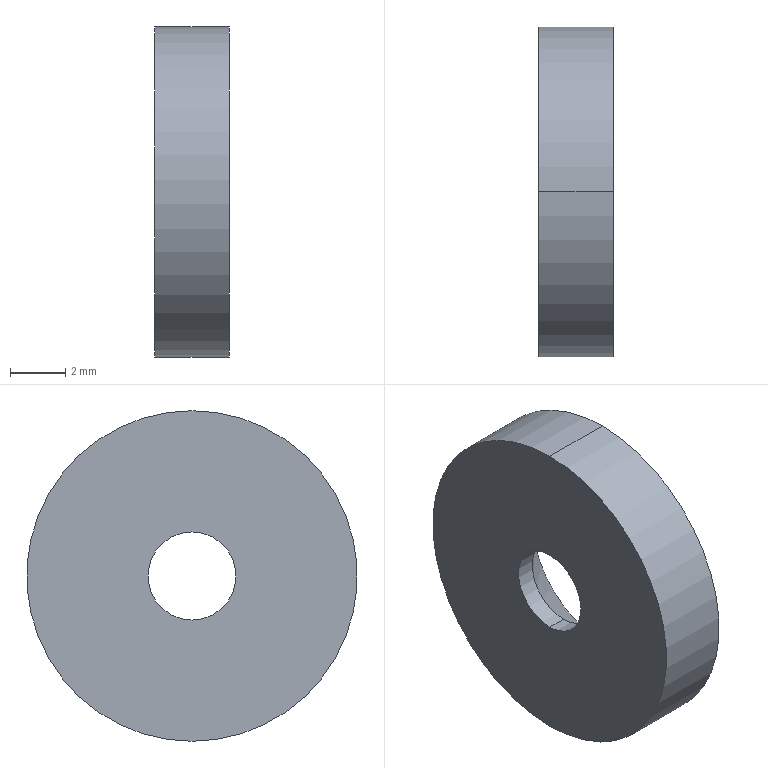Part | STEP file | NdFeB round magnet D12X3 with 3mm hole | 1 solid | 8 faces | box 2.7 x 12 x 12 mm | volume 255.164 mm3 | cylinder 4 | cone 2 | plane 2 | commonest cylinder face diameters 3.2 x2 12 x2
STEP:
#1=CARTESIAN_POINT('',(0.,0.,0.));
#2=DIRECTION('',(0.,0.,1.));
#3=DIRECTION('',(1.,0.,0.));
#4=AXIS2_PLACEMENT_3D('',#1,#2,#3);
#5=CARTESIAN_POINT('',(0.7,0.,-1.6));
#6=VERTEX_POINT('',#5);
#7=CARTESIAN_POINT('',(2.7,0.,-3.6));
#8=VERTEX_POINT('',#7);
#9=CARTESIAN_POINT('',(0.7,0.,-1.6));
#10=DIRECTION('',(0.7071,0.,-0.7071));
#11=VECTOR('',#10,1.);
#12=LINE('',#9,#11);
#13=CARTESIAN_POINT('',(0.7,0.,0.));
#14=DIRECTION('',(1.,0.,0.));
#15=DIRECTION('',(0.,0.,-1.));
#16=AXIS2_PLACEMENT_3D('',#13,#14,#15);
#17=CONICAL_SURFACE('',#16,1.6,0.7854);
#18=CARTESIAN_POINT('',(6.283,0.));
#19=DIRECTION('',(0.,1.));
#20=VECTOR('',#19,1.);
#21=LINE('',#18,#20);
#22=(GEOMETRIC_REPRESENTATION_CONTEXT(2)PARAMETRIC_REPRESENTATION_CONTEXT()REPRESENTATION_CONTEXT('',''));
#23=DEFINITIONAL_REPRESENTATION('',(#21),#22);
#24=PCURVE('',#17,#23);
#25=CARTESIAN_POINT('',(0.7,0.,0.));
#26=DIRECTION('',(1.,0.,0.));
#27=DIRECTION('',(0.,0.,-1.));
#28=AXIS2_PLACEMENT_3D('',#25,#26,#27);
#29=CONICAL_SURFACE('',#28,1.6,0.7854);
#30=CARTESIAN_POINT('',(0.,0.));
#31=DIRECTION('',(0.,1.));
#32=VECTOR('',#31,1.);
#33=LINE('',#30,#32);
#34=(GEOMETRIC_REPRESENTATION_CONTEXT(2)PARAMETRIC_REPRESENTATION_CONTEXT()REPRESENTATION_CONTEXT('',''));
#35=DEFINITIONAL_REPRESENTATION('',(#33),#34);
#36=PCURVE('',#29,#35);
#37=SURFACE_CURVE('',#12,(#24,#36),.PCURVE_S1.);
#38=EDGE_CURVE('',#6,#8,#37,.T.);
#39=ORIENTED_EDGE('',*,*,#38,.T.);
#40=CARTESIAN_POINT('',(2.7,0.,3.6));
#41=VERTEX_POINT('',#40);
#42=CARTESIAN_POINT('',(2.7,0.,0.));
#43=DIRECTION('',(-1.,0.,0.));
#44=DIRECTION('',(0.,0.,-1.));
#45=AXIS2_PLACEMENT_3D('',#42,#43,#44);
#46=CIRCLE('',#45,3.6);
#47=CARTESIAN_POINT('',(6.283,2.));
#48=DIRECTION('',(-1.,0.));
#49=VECTOR('',#48,1.);
#50=LINE('',#47,#49);
#51=(GEOMETRIC_REPRESENTATION_CONTEXT(2)PARAMETRIC_REPRESENTATION_CONTEXT()REPRESENTATION_CONTEXT('',''));
#52=DEFINITIONAL_REPRESENTATION('',(#50),#51);
#53=PCURVE('',#17,#52);
#54=CARTESIAN_POINT('',(2.7,0.,0.));
#55=DIRECTION('',(1.,0.,0.));
#56=DIRECTION('',(0.,0.,-1.));
#57=AXIS2_PLACEMENT_3D('',#54,#55,#56);
#58=PLANE('',#57);
#59=CARTESIAN_POINT('',(3.6,0.));
#60=CARTESIAN_POINT('',(3.6,-6.235));
#61=CARTESIAN_POINT('',(-1.8,-3.118));
#62=CARTESIAN_POINT('',(-7.2,0.));
#63=CARTESIAN_POINT('',(-1.8,3.118));
#64=CARTESIAN_POINT('',(3.6,6.235));
#65=CARTESIAN_POINT('',(3.6,0.));
#66=(BOUNDED_CURVE()B_SPLINE_CURVE(2,(#59,#60,#61,#62,#63,#64,#65),.UNSPECIFIED.,.T.,.F.)B_SPLINE_CURVE_WITH_KNOTS((1,2,2,2,2,1),(-2.094,0.,2.094,4.189,6.283,8.378),.UNSPECIFIED.)CURVE()GEOMETRIC_REPRESENTATION_ITEM()RATIONAL_B_SPLINE_CURVE((1.,0.5,1.,0.5,1.,0.5,1.))REPRESENTATION_ITEM(''));
#67=(GEOMETRIC_REPRESENTATION_CONTEXT(2)PARAMETRIC_REPRESENTATION_CONTEXT()REPRESENTATION_CONTEXT('',''));
#68=DEFINITIONAL_REPRESENTATION('',(#66),#67);
#69=PCURVE('',#58,#68);
#70=SURFACE_CURVE('',#46,(#53,#69),.PCURVE_S1.);
#71=EDGE_CURVE('',#8,#41,#70,.T.);
#72=ORIENTED_EDGE('',*,*,#71,.T.);
#73=CARTESIAN_POINT('',(0.7,0.,1.6));
#74=VERTEX_POINT('',#73);
#75=CARTESIAN_POINT('',(0.7,0.,1.6));
#76=DIRECTION('',(0.7071,0.,0.7071));
#77=VECTOR('',#76,1.);
#78=LINE('',#75,#77);
#79=CARTESIAN_POINT('',(3.142,0.));
#80=DIRECTION('',(0.,1.));
#81=VECTOR('',#80,1.);
#82=LINE('',#79,#81);
#83=(GEOMETRIC_REPRESENTATION_CONTEXT(2)PARAMETRIC_REPRESENTATION_CONTEXT()REPRESENTATION_CONTEXT('',''));
#84=DEFINITIONAL_REPRESENTATION('',(#82),#83);
#85=PCURVE('',#17,#84);
#86=CARTESIAN_POINT('',(3.142,0.));
#87=DIRECTION('',(0.,1.));
#88=VECTOR('',#87,1.);
#89=LINE('',#86,#88);
#90=(GEOMETRIC_REPRESENTATION_CONTEXT(2)PARAMETRIC_REPRESENTATION_CONTEXT()REPRESENTATION_CONTEXT('',''));
#91=DEFINITIONAL_REPRESENTATION('',(#89),#90);
#92=PCURVE('',#29,#91);
#93=SURFACE_CURVE('',#78,(#85,#92),.PCURVE_S1.);
#94=EDGE_CURVE('',#74,#41,#93,.T.);
#95=ORIENTED_EDGE('',*,*,#94,.F.);
#96=CARTESIAN_POINT('',(0.7,0.,0.));
#97=DIRECTION('',(1.,0.,0.));
#98=DIRECTION('',(0.,0.,-1.));
#99=AXIS2_PLACEMENT_3D('',#96,#97,#98);
#100=CIRCLE('',#99,1.6);
#101=CARTESIAN_POINT('',(0.,0.));
#102=DIRECTION('',(1.,0.));
#103=VECTOR('',#102,1.);
#104=LINE('',#101,#103);
#105=(GEOMETRIC_REPRESENTATION_CONTEXT(2)PARAMETRIC_REPRESENTATION_CONTEXT()REPRESENTATION_CONTEXT('',''));
#106=DEFINITIONAL_REPRESENTATION('',(#104),#105);
#107=PCURVE('',#17,#106);
#108=CARTESIAN_POINT('',(2.7,0.,0.));
#109=DIRECTION('',(-1.,0.,0.));
#110=DIRECTION('',(0.,0.,1.));
#111=AXIS2_PLACEMENT_3D('',#108,#109,#110);
#112=CYLINDRICAL_SURFACE('',#111,1.6);
#113=CARTESIAN_POINT('',(9.425,2.));
#114=DIRECTION('',(-1.,0.));
#115=VECTOR('',#114,1.);
#116=LINE('',#113,#115);
#117=(GEOMETRIC_REPRESENTATION_CONTEXT(2)PARAMETRIC_REPRESENTATION_CONTEXT()REPRESENTATION_CONTEXT('',''));
#118=DEFINITIONAL_REPRESENTATION('',(#116),#117);
#119=PCURVE('',#112,#118);
#120=SURFACE_CURVE('',#100,(#107,#119),.PCURVE_S1.);
#121=EDGE_CURVE('',#74,#6,#120,.T.);
#122=ORIENTED_EDGE('',*,*,#121,.T.);
#123=EDGE_LOOP('',(#39,#72,#95,#122));
#124=FACE_BOUND('',#123,.F.);
#125=ADVANCED_FACE('',(#124),#17,.F.);
#126=CARTESIAN_POINT('',(0.,0.,1.6));
#127=VERTEX_POINT('',#126);
#128=CARTESIAN_POINT('',(2.7,0.,1.6));
#129=DIRECTION('',(-1.,0.,0.));
#130=VECTOR('',#129,1.);
#131=LINE('',#128,#130);
#132=CARTESIAN_POINT('',(6.283,0.));
#133=DIRECTION('',(0.,1.));
#134=VECTOR('',#133,1.);
#135=LINE('',#132,#134);
#136=(GEOMETRIC_REPRESENTATION_CONTEXT(2)PARAMETRIC_REPRESENTATION_CONTEXT()REPRESENTATION_CONTEXT('',''));
#137=DEFINITIONAL_REPRESENTATION('',(#135),#136);
#138=PCURVE('',#112,#137);
#139=CARTESIAN_POINT('',(2.7,0.,0.));
#140=DIRECTION('',(-1.,0.,0.));
#141=DIRECTION('',(0.,0.,1.));
#142=AXIS2_PLACEMENT_3D('',#139,#140,#141);
#143=CYLINDRICAL_SURFACE('',#142,1.6);
#144=CARTESIAN_POINT('',(0.,0.));
#145=DIRECTION('',(0.,1.));
#146=VECTOR('',#145,1.);
#147=LINE('',#144,#146);
#148=(GEOMETRIC_REPRESENTATION_CONTEXT(2)PARAMETRIC_REPRESENTATION_CONTEXT()REPRESENTATION_CONTEXT('',''));
#149=DEFINITIONAL_REPRESENTATION('',(#147),#148);
#150=PCURVE('',#143,#149);
#151=SURFACE_CURVE('',#131,(#138,#150),.PCURVE_S1.);
#152=EDGE_CURVE('',#74,#127,#151,.T.);
#153=ORIENTED_EDGE('',*,*,#152,.T.);
#154=CARTESIAN_POINT('',(0.,0.,-1.6));
#155=VERTEX_POINT('',#154);
#156=CARTESIAN_POINT('',(0.,0.,0.));
#157=DIRECTION('',(1.,0.,0.));
#158=DIRECTION('',(0.,0.,-1.));
#159=AXIS2_PLACEMENT_3D('',#156,#157,#158);
#160=CIRCLE('',#159,1.6);
#161=CARTESIAN_POINT('',(9.425,2.7));
#162=DIRECTION('',(-1.,0.));
#163=VECTOR('',#162,1.);
#164=LINE('',#161,#163);
#165=(GEOMETRIC_REPRESENTATION_CONTEXT(2)PARAMETRIC_REPRESENTATION_CONTEXT()REPRESENTATION_CONTEXT('',''));
#166=DEFINITIONAL_REPRESENTATION('',(#164),#165);
#167=PCURVE('',#112,#166);
#168=CARTESIAN_POINT('',(0.,0.,0.));
#169=DIRECTION('',(1.,0.,0.));
#170=DIRECTION('',(0.,0.,-1.));
#171=AXIS2_PLACEMENT_3D('',#168,#169,#170);
#172=PLANE('',#171);
#173=CARTESIAN_POINT('',(0.,0.));
#174=DIRECTION('',(1.,0.));
#175=AXIS2_PLACEMENT_2D('',#173,#174);
#176=CIRCLE('',#175,1.6);
#177=(GEOMETRIC_REPRESENTATION_CONTEXT(2)PARAMETRIC_REPRESENTATION_CONTEXT()REPRESENTATION_CONTEXT('',''));
#178=DEFINITIONAL_REPRESENTATION('',(#176),#177);
#179=PCURVE('',#172,#178);
#180=SURFACE_CURVE('',#160,(#167,#179),.PCURVE_S1.);
#181=EDGE_CURVE('',#127,#155,#180,.T.);
#182=ORIENTED_EDGE('',*,*,#181,.T.);
#183=CARTESIAN_POINT('',(2.7,0.,-1.6));
#184=DIRECTION('',(-1.,0.,0.));
#185=VECTOR('',#184,1.);
#186=LINE('',#183,#185);
#187=CARTESIAN_POINT('',(3.142,0.));
#188=DIRECTION('',(0.,1.));
#189=VECTOR('',#188,1.);
#190=LINE('',#187,#189);
#191=(GEOMETRIC_REPRESENTATION_CONTEXT(2)PARAMETRIC_REPRESENTATION_CONTEXT()REPRESENTATION_CONTEXT('',''));
#192=DEFINITIONAL_REPRESENTATION('',(#190),#191);
#193=PCURVE('',#112,#192);
#194=CARTESIAN_POINT('',(3.142,0.));
#195=DIRECTION('',(0.,1.));
#196=VECTOR('',#195,1.);
#197=LINE('',#194,#196);
#198=(GEOMETRIC_REPRESENTATION_CONTEXT(2)PARAMETRIC_REPRESENTATION_CONTEXT()REPRESENTATION_CONTEXT('',''));
#199=DEFINITIONAL_REPRESENTATION('',(#197),#198);
#200=PCURVE('',#143,#199);
#201=SURFACE_CURVE('',#186,(#193,#200),.PCURVE_S1.);
#202=EDGE_CURVE('',#6,#155,#201,.T.);
#203=ORIENTED_EDGE('',*,*,#202,.F.);
#204=ORIENTED_EDGE('',*,*,#121,.F.);
#205=EDGE_LOOP('',(#153,#182,#203,#204));
#206=FACE_BOUND('',#205,.F.);
#207=ADVANCED_FACE('',(#206),#112,.F.);
#208=CARTESIAN_POINT('',(2.7,0.,-6.));
#209=VERTEX_POINT('',#208);
#210=CARTESIAN_POINT('',(2.7,0.,6.));
#211=VERTEX_POINT('',#210);
#212=CARTESIAN_POINT('',(2.7,0.,0.));
#213=DIRECTION('',(1.,0.,0.));
#214=DIRECTION('',(0.,0.,-1.));
#215=AXIS2_PLACEMENT_3D('',#212,#213,#214);
#216=CIRCLE('',#215,6.);
#217=CARTESIAN_POINT('',(2.7,0.,0.));
#218=DIRECTION('',(-1.,0.,0.));
#219=DIRECTION('',(0.,0.,1.));
#220=AXIS2_PLACEMENT_3D('',#217,#218,#219);
#221=CYLINDRICAL_SURFACE('',#220,6.);
#222=CARTESIAN_POINT('',(3.142,0.));
#223=DIRECTION('',(-1.,0.));
#224=VECTOR('',#223,1.);
#225=LINE('',#222,#224);
#226=(GEOMETRIC_REPRESENTATION_CONTEXT(2)PARAMETRIC_REPRESENTATION_CONTEXT()REPRESENTATION_CONTEXT('',''));
#227=DEFINITIONAL_REPRESENTATION('',(#225),#226);
#228=PCURVE('',#221,#227);
#229=CARTESIAN_POINT('',(0.,0.));
#230=DIRECTION('',(1.,0.));
#231=AXIS2_PLACEMENT_2D('',#229,#230);
#232=CIRCLE('',#231,6.);
#233=(GEOMETRIC_REPRESENTATION_CONTEXT(2)PARAMETRIC_REPRESENTATION_CONTEXT()REPRESENTATION_CONTEXT('',''));
#234=DEFINITIONAL_REPRESENTATION('',(#232),#233);
#235=PCURVE('',#58,#234);
#236=SURFACE_CURVE('',#216,(#228,#235),.PCURVE_S1.);
#237=EDGE_CURVE('',#209,#211,#236,.T.);
#238=ORIENTED_EDGE('',*,*,#237,.F.);
#239=CARTESIAN_POINT('',(0.,0.,-6.));
#240=VERTEX_POINT('',#239);
#241=CARTESIAN_POINT('',(2.7,0.,-6.));
#242=DIRECTION('',(-1.,0.,0.));
#243=VECTOR('',#242,1.);
#244=LINE('',#241,#243);
#245=CARTESIAN_POINT('',(3.142,0.));
#246=DIRECTION('',(0.,1.));
#247=VECTOR('',#246,1.);
#248=LINE('',#245,#247);
#249=(GEOMETRIC_REPRESENTATION_CONTEXT(2)PARAMETRIC_REPRESENTATION_CONTEXT()REPRESENTATION_CONTEXT('',''));
#250=DEFINITIONAL_REPRESENTATION('',(#248),#249);
#251=PCURVE('',#221,#250);
#252=CARTESIAN_POINT('',(2.7,0.,0.));
#253=DIRECTION('',(-1.,0.,0.));
#254=DIRECTION('',(0.,0.,1.));
#255=AXIS2_PLACEMENT_3D('',#252,#253,#254);
#256=CYLINDRICAL_SURFACE('',#255,6.);
#257=CARTESIAN_POINT('',(3.142,0.));
#258=DIRECTION('',(0.,1.));
#259=VECTOR('',#258,1.);
#260=LINE('',#257,#259);
#261=(GEOMETRIC_REPRESENTATION_CONTEXT(2)PARAMETRIC_REPRESENTATION_CONTEXT()REPRESENTATION_CONTEXT('',''));
#262=DEFINITIONAL_REPRESENTATION('',(#260),#261);
#263=PCURVE('',#256,#262);
#264=SURFACE_CURVE('',#244,(#251,#263),.PCURVE_S1.);
#265=EDGE_CURVE('',#209,#240,#264,.T.);
#266=ORIENTED_EDGE('',*,*,#265,.T.);
#267=CARTESIAN_POINT('',(0.,0.,6.));
#268=VERTEX_POINT('',#267);
#269=CARTESIAN_POINT('',(0.,0.,0.));
#270=DIRECTION('',(1.,0.,0.));
#271=DIRECTION('',(0.,0.,-1.));
#272=AXIS2_PLACEMENT_3D('',#269,#270,#271);
#273=CIRCLE('',#272,6.);
#274=CARTESIAN_POINT('',(3.142,2.7));
#275=DIRECTION('',(-1.,0.));
#276=VECTOR('',#275,1.);
#277=LINE('',#274,#276);
#278=(GEOMETRIC_REPRESENTATION_CONTEXT(2)PARAMETRIC_REPRESENTATION_CONTEXT()REPRESENTATION_CONTEXT('',''));
#279=DEFINITIONAL_REPRESENTATION('',(#277),#278);
#280=PCURVE('',#221,#279);
#281=CARTESIAN_POINT('',(0.,0.));
#282=DIRECTION('',(1.,0.));
#283=AXIS2_PLACEMENT_2D('',#281,#282);
#284=CIRCLE('',#283,6.);
#285=(GEOMETRIC_REPRESENTATION_CONTEXT(2)PARAMETRIC_REPRESENTATION_CONTEXT()REPRESENTATION_CONTEXT('',''));
#286=DEFINITIONAL_REPRESENTATION('',(#284),#285);
#287=PCURVE('',#172,#286);
#288=SURFACE_CURVE('',#273,(#280,#287),.PCURVE_S1.);
#289=EDGE_CURVE('',#240,#268,#288,.T.);
#290=ORIENTED_EDGE('',*,*,#289,.T.);
#291=CARTESIAN_POINT('',(2.7,0.,6.));
#292=DIRECTION('',(-1.,0.,0.));
#293=VECTOR('',#292,1.);
#294=LINE('',#291,#293);
#295=CARTESIAN_POINT('',(0.,0.));
#296=DIRECTION('',(0.,1.));
#297=VECTOR('',#296,1.);
#298=LINE('',#295,#297);
#299=(GEOMETRIC_REPRESENTATION_CONTEXT(2)PARAMETRIC_REPRESENTATION_CONTEXT()REPRESENTATION_CONTEXT('',''));
#300=DEFINITIONAL_REPRESENTATION('',(#298),#299);
#301=PCURVE('',#221,#300);
#302=CARTESIAN_POINT('',(6.283,0.));
#303=DIRECTION('',(0.,1.));
#304=VECTOR('',#303,1.);
#305=LINE('',#302,#304);
#306=(GEOMETRIC_REPRESENTATION_CONTEXT(2)PARAMETRIC_REPRESENTATION_CONTEXT()REPRESENTATION_CONTEXT('',''));
#307=DEFINITIONAL_REPRESENTATION('',(#305),#306);
#308=PCURVE('',#256,#307);
#309=SURFACE_CURVE('',#294,(#301,#308),.PCURVE_S1.);
#310=EDGE_CURVE('',#211,#268,#309,.T.);
#311=ORIENTED_EDGE('',*,*,#310,.F.);
#312=EDGE_LOOP('',(#238,#266,#290,#311));
#313=FACE_BOUND('',#312,.T.);
#314=ADVANCED_FACE('',(#313),#221,.T.);
#315=ORIENTED_EDGE('',*,*,#71,.T.);
#316=CARTESIAN_POINT('',(2.7,0.,0.));
#317=DIRECTION('',(-1.,0.,0.));
#318=DIRECTION('',(0.,0.,-1.));
#319=AXIS2_PLACEMENT_3D('',#316,#317,#318);
#320=CIRCLE('',#319,3.6);
#321=CARTESIAN_POINT('',(3.6,0.));
#322=CARTESIAN_POINT('',(3.6,-6.235));
#323=CARTESIAN_POINT('',(-1.8,-3.118));
#324=CARTESIAN_POINT('',(-7.2,0.));
#325=CARTESIAN_POINT('',(-1.8,3.118));
#326=CARTESIAN_POINT('',(3.6,6.235));
#327=CARTESIAN_POINT('',(3.6,0.));
#328=(BOUNDED_CURVE()B_SPLINE_CURVE(2,(#321,#322,#323,#324,#325,#326,#327),.UNSPECIFIED.,.T.,.F.)B_SPLINE_CURVE_WITH_KNOTS((1,2,2,2,2,1),(-2.094,0.,2.094,4.189,6.283,8.378),.UNSPECIFIED.)CURVE()GEOMETRIC_REPRESENTATION_ITEM()RATIONAL_B_SPLINE_CURVE((1.,0.5,1.,0.5,1.,0.5,1.))REPRESENTATION_ITEM(''));
#329=(GEOMETRIC_REPRESENTATION_CONTEXT(2)PARAMETRIC_REPRESENTATION_CONTEXT()REPRESENTATION_CONTEXT('',''));
#330=DEFINITIONAL_REPRESENTATION('',(#328),#329);
#331=PCURVE('',#58,#330);
#332=CARTESIAN_POINT('',(6.283,2.));
#333=DIRECTION('',(-1.,0.));
#334=VECTOR('',#333,1.);
#335=LINE('',#332,#334);
#336=(GEOMETRIC_REPRESENTATION_CONTEXT(2)PARAMETRIC_REPRESENTATION_CONTEXT()REPRESENTATION_CONTEXT('',''));
#337=DEFINITIONAL_REPRESENTATION('',(#335),#336);
#338=PCURVE('',#29,#337);
#339=SURFACE_CURVE('',#320,(#331,#338),.PCURVE_S1.);
#340=EDGE_CURVE('',#41,#8,#339,.T.);
#341=ORIENTED_EDGE('',*,*,#340,.T.);
#342=EDGE_LOOP('',(#315,#341));
#343=FACE_BOUND('',#342,.T.);
#344=CARTESIAN_POINT('',(2.7,0.,0.));
#345=DIRECTION('',(1.,0.,0.));
#346=DIRECTION('',(0.,0.,-1.));
#347=AXIS2_PLACEMENT_3D('',#344,#345,#346);
#348=CIRCLE('',#347,6.);
#349=CARTESIAN_POINT('',(0.,0.));
#350=DIRECTION('',(1.,0.));
#351=AXIS2_PLACEMENT_2D('',#349,#350);
#352=CIRCLE('',#351,6.);
#353=(GEOMETRIC_REPRESENTATION_CONTEXT(2)PARAMETRIC_REPRESENTATION_CONTEXT()REPRESENTATION_CONTEXT('',''));
#354=DEFINITIONAL_REPRESENTATION('',(#352),#353);
#355=PCURVE('',#58,#354);
#356=CARTESIAN_POINT('',(9.425,0.));
#357=DIRECTION('',(-1.,0.));
#358=VECTOR('',#357,1.);
#359=LINE('',#356,#358);
#360=(GEOMETRIC_REPRESENTATION_CONTEXT(2)PARAMETRIC_REPRESENTATION_CONTEXT()REPRESENTATION_CONTEXT('',''));
#361=DEFINITIONAL_REPRESENTATION('',(#359),#360);
#362=PCURVE('',#256,#361);
#363=SURFACE_CURVE('',#348,(#355,#362),.PCURVE_S1.);
#364=EDGE_CURVE('',#211,#209,#363,.T.);
#365=ORIENTED_EDGE('',*,*,#364,.T.);
#366=ORIENTED_EDGE('',*,*,#237,.T.);
#367=EDGE_LOOP('',(#365,#366));
#368=FACE_BOUND('',#367,.T.);
#369=ADVANCED_FACE('',(#343,#368),#58,.T.);
#370=CARTESIAN_POINT('',(0.,0.,0.));
#371=DIRECTION('',(1.,0.,0.));
#372=DIRECTION('',(0.,0.,-1.));
#373=AXIS2_PLACEMENT_3D('',#370,#371,#372);
#374=CIRCLE('',#373,6.);
#375=CARTESIAN_POINT('',(0.,0.));
#376=DIRECTION('',(1.,0.));
#377=AXIS2_PLACEMENT_2D('',#375,#376);
#378=CIRCLE('',#377,6.);
#379=(GEOMETRIC_REPRESENTATION_CONTEXT(2)PARAMETRIC_REPRESENTATION_CONTEXT()REPRESENTATION_CONTEXT('',''));
#380=DEFINITIONAL_REPRESENTATION('',(#378),#379);
#381=PCURVE('',#172,#380);
#382=CARTESIAN_POINT('',(9.425,2.7));
#383=DIRECTION('',(-1.,0.));
#384=VECTOR('',#383,1.);
#385=LINE('',#382,#384);
#386=(GEOMETRIC_REPRESENTATION_CONTEXT(2)PARAMETRIC_REPRESENTATION_CONTEXT()REPRESENTATION_CONTEXT('',''));
#387=DEFINITIONAL_REPRESENTATION('',(#385),#386);
#388=PCURVE('',#256,#387);
#389=SURFACE_CURVE('',#374,(#381,#388),.PCURVE_S1.);
#390=EDGE_CURVE('',#268,#240,#389,.T.);
#391=ORIENTED_EDGE('',*,*,#390,.F.);
#392=ORIENTED_EDGE('',*,*,#289,.F.);
#393=EDGE_LOOP('',(#391,#392));
#394=FACE_BOUND('',#393,.T.);
#395=ORIENTED_EDGE('',*,*,#181,.T.);
#396=CARTESIAN_POINT('',(0.,0.,0.));
#397=DIRECTION('',(1.,0.,0.));
#398=DIRECTION('',(0.,0.,-1.));
#399=AXIS2_PLACEMENT_3D('',#396,#397,#398);
#400=CIRCLE('',#399,1.6);
#401=CARTESIAN_POINT('',(0.,0.));
#402=DIRECTION('',(1.,0.));
#403=AXIS2_PLACEMENT_2D('',#401,#402);
#404=CIRCLE('',#403,1.6);
#405=(GEOMETRIC_REPRESENTATION_CONTEXT(2)PARAMETRIC_REPRESENTATION_CONTEXT()REPRESENTATION_CONTEXT('',''));
#406=DEFINITIONAL_REPRESENTATION('',(#404),#405);
#407=PCURVE('',#172,#406);
#408=CARTESIAN_POINT('',(3.142,2.7));
#409=DIRECTION('',(-1.,0.));
#410=VECTOR('',#409,1.);
#411=LINE('',#408,#410);
#412=(GEOMETRIC_REPRESENTATION_CONTEXT(2)PARAMETRIC_REPRESENTATION_CONTEXT()REPRESENTATION_CONTEXT('',''));
#413=DEFINITIONAL_REPRESENTATION('',(#411),#412);
#414=PCURVE('',#143,#413);
#415=SURFACE_CURVE('',#400,(#407,#414),.PCURVE_S1.);
#416=EDGE_CURVE('',#155,#127,#415,.T.);
#417=ORIENTED_EDGE('',*,*,#416,.T.);
#418=EDGE_LOOP('',(#395,#417));
#419=FACE_BOUND('',#418,.T.);
#420=ADVANCED_FACE('',(#394,#419),#172,.F.);
#421=ORIENTED_EDGE('',*,*,#265,.F.);
#422=ORIENTED_EDGE('',*,*,#364,.F.);
#423=ORIENTED_EDGE('',*,*,#310,.T.);
#424=ORIENTED_EDGE('',*,*,#390,.T.);
#425=EDGE_LOOP('',(#421,#422,#423,#424));
#426=FACE_BOUND('',#425,.T.);
#427=ADVANCED_FACE('',(#426),#256,.T.);
#428=ORIENTED_EDGE('',*,*,#416,.T.);
#429=ORIENTED_EDGE('',*,*,#152,.F.);
#430=CARTESIAN_POINT('',(0.7,0.,0.));
#431=DIRECTION('',(1.,0.,0.));
#432=DIRECTION('',(0.,0.,-1.));
#433=AXIS2_PLACEMENT_3D('',#430,#431,#432);
#434=CIRCLE('',#433,1.6);
#435=CARTESIAN_POINT('',(3.142,2.));
#436=DIRECTION('',(-1.,0.));
#437=VECTOR('',#436,1.);
#438=LINE('',#435,#437);
#439=(GEOMETRIC_REPRESENTATION_CONTEXT(2)PARAMETRIC_REPRESENTATION_CONTEXT()REPRESENTATION_CONTEXT('',''));
#440=DEFINITIONAL_REPRESENTATION('',(#438),#439);
#441=PCURVE('',#143,#440);
#442=CARTESIAN_POINT('',(0.,0.));
#443=DIRECTION('',(1.,0.));
#444=VECTOR('',#443,1.);
#445=LINE('',#442,#444);
#446=(GEOMETRIC_REPRESENTATION_CONTEXT(2)PARAMETRIC_REPRESENTATION_CONTEXT()REPRESENTATION_CONTEXT('',''));
#447=DEFINITIONAL_REPRESENTATION('',(#445),#446);
#448=PCURVE('',#29,#447);
#449=SURFACE_CURVE('',#434,(#441,#448),.PCURVE_S1.);
#450=EDGE_CURVE('',#6,#74,#449,.T.);
#451=ORIENTED_EDGE('',*,*,#450,.F.);
#452=ORIENTED_EDGE('',*,*,#202,.T.);
#453=EDGE_LOOP('',(#428,#429,#451,#452));
#454=FACE_BOUND('',#453,.F.);
#455=ADVANCED_FACE('',(#454),#143,.F.);
#456=ORIENTED_EDGE('',*,*,#340,.T.);
#457=ORIENTED_EDGE('',*,*,#38,.F.);
#458=ORIENTED_EDGE('',*,*,#450,.T.);
#459=ORIENTED_EDGE('',*,*,#94,.T.);
#460=EDGE_LOOP('',(#456,#457,#458,#459));
#461=FACE_BOUND('',#460,.F.);
#462=ADVANCED_FACE('',(#461),#29,.F.);
#463=CLOSED_SHELL('',(#125,#207,#314,#369,#420,#427,#455,#462));
#464=MANIFOLD_SOLID_BREP('',#463);
#465=(LENGTH_UNIT()NAMED_UNIT(*)SI_UNIT(.MILLI.,.METRE.));
#466=UNCERTAINTY_MEASURE_WITH_UNIT(LENGTH_MEASURE(0.0000001),#465,'','');
#467=(NAMED_UNIT(*)PLANE_ANGLE_UNIT()SI_UNIT($,.RADIAN.));
#468=(NAMED_UNIT(*)SI_UNIT($,.STERADIAN.)SOLID_ANGLE_UNIT());
#469=(GEOMETRIC_REPRESENTATION_CONTEXT(3)GLOBAL_UNCERTAINTY_ASSIGNED_CONTEXT((#466))GLOBAL_UNIT_ASSIGNED_CONTEXT((#465,#467,#468))REPRESENTATION_CONTEXT('',''));
#470=ADVANCED_BREP_SHAPE_REPRESENTATION('',(#4,#464),#469);